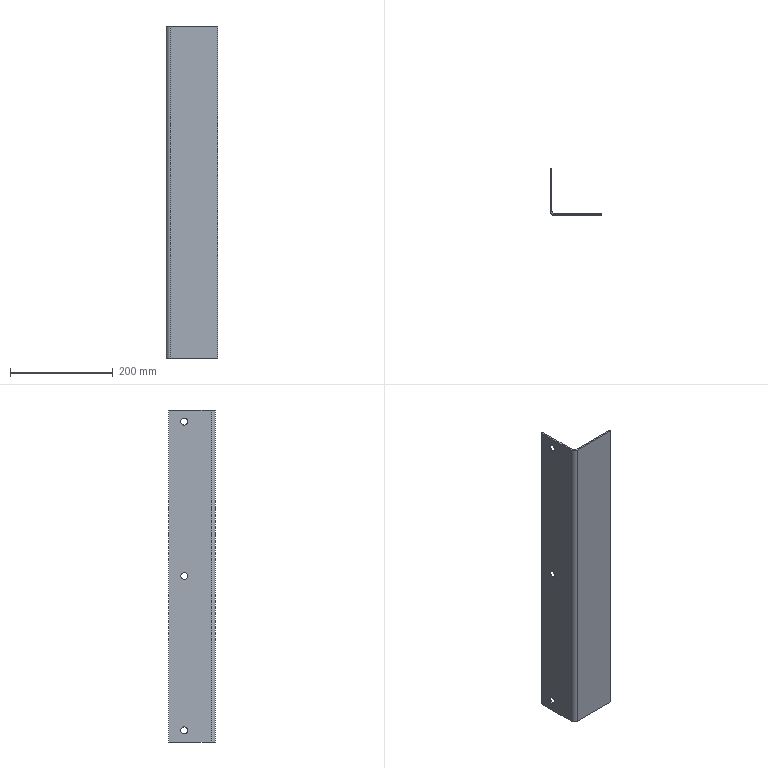Part | SolidWorks | features FlatPattern 1, ICE 1, SMBaseFlange 1, SheetMetal 1 | 1 solid | 20 faces | box 100 x 90 x 645 mm | volume 355061 mm3 | plane 12 | cylinder 8 | commonest cylinder face diameters 14 x6 10 x1 16 x1
STEP:
#1=CARTESIAN_POINT('',(0.,67.,300.));
#2=VERTEX_POINT('',#1);
#3=CARTESIAN_POINT('',(0.,53.,300.));
#4=VERTEX_POINT('',#3);
#5=CARTESIAN_POINT('',(0.,60.,300.));
#6=DIRECTION('',(-1.,0.,0.));
#7=DIRECTION('',(0.,-1.,0.));
#8=AXIS2_PLACEMENT_3D('',#5,#6,#7);
#9=CIRCLE('',#8,7.);
#10=EDGE_CURVE('',#2,#4,#9,.T.);
#11=ORIENTED_EDGE('',*,*,#10,.T.);
#12=CARTESIAN_POINT('',(3.,53.,300.));
#13=VERTEX_POINT('',#12);
#14=CARTESIAN_POINT('',(-7.,53.,300.));
#15=DIRECTION('',(1.,0.,0.));
#16=VECTOR('',#15,1000.);
#17=LINE('',#14,#16);
#18=EDGE_CURVE('',#4,#13,#17,.T.);
#19=ORIENTED_EDGE('',*,*,#18,.T.);
#20=CARTESIAN_POINT('',(3.,67.,300.));
#21=VERTEX_POINT('',#20);
#22=CARTESIAN_POINT('',(3.,60.,300.));
#23=DIRECTION('',(1.,0.,0.));
#24=DIRECTION('',(0.,1.,0.));
#25=AXIS2_PLACEMENT_3D('',#22,#23,#24);
#26=CIRCLE('',#25,7.);
#27=EDGE_CURVE('',#13,#21,#26,.T.);
#28=ORIENTED_EDGE('',*,*,#27,.T.);
#29=CARTESIAN_POINT('',(-7.,67.,300.));
#30=DIRECTION('',(1.,0.,0.));
#31=VECTOR('',#30,1000.);
#32=LINE('',#29,#31);
#33=EDGE_CURVE('',#2,#21,#32,.T.);
#34=ORIENTED_EDGE('',*,*,#33,.F.);
#35=EDGE_LOOP('',(#11,#19,#28,#34));
#36=FACE_OUTER_BOUND('',#35,.T.);
#37=CARTESIAN_POINT('',(-7.,60.,300.));
#38=DIRECTION('',(1.,0.,0.));
#39=DIRECTION('',(0.,1.,0.));
#40=AXIS2_PLACEMENT_3D('',#37,#38,#39);
#41=CYLINDRICAL_SURFACE('',#40,7.);
#42=ADVANCED_FACE('',(#36),#41,.F.);
#43=CARTESIAN_POINT('',(0.,67.,-300.));
#44=VERTEX_POINT('',#43);
#45=CARTESIAN_POINT('',(0.,53.,-300.));
#46=VERTEX_POINT('',#45);
#47=CARTESIAN_POINT('',(0.,60.,-300.));
#48=DIRECTION('',(-1.,0.,0.));
#49=DIRECTION('',(0.,-1.,0.));
#50=AXIS2_PLACEMENT_3D('',#47,#48,#49);
#51=CIRCLE('',#50,7.);
#52=EDGE_CURVE('',#44,#46,#51,.T.);
#53=ORIENTED_EDGE('',*,*,#52,.T.);
#54=CARTESIAN_POINT('',(3.,53.,-300.));
#55=VERTEX_POINT('',#54);
#56=CARTESIAN_POINT('',(-7.,53.,-300.));
#57=DIRECTION('',(1.,0.,0.));
#58=VECTOR('',#57,1000.);
#59=LINE('',#56,#58);
#60=EDGE_CURVE('',#46,#55,#59,.T.);
#61=ORIENTED_EDGE('',*,*,#60,.T.);
#62=CARTESIAN_POINT('',(3.,67.,-300.));
#63=VERTEX_POINT('',#62);
#64=CARTESIAN_POINT('',(3.,60.,-300.));
#65=DIRECTION('',(1.,0.,0.));
#66=DIRECTION('',(0.,1.,0.));
#67=AXIS2_PLACEMENT_3D('',#64,#65,#66);
#68=CIRCLE('',#67,7.);
#69=EDGE_CURVE('',#55,#63,#68,.T.);
#70=ORIENTED_EDGE('',*,*,#69,.T.);
#71=CARTESIAN_POINT('',(-7.,67.,-300.));
#72=DIRECTION('',(1.,0.,0.));
#73=VECTOR('',#72,1000.);
#74=LINE('',#71,#73);
#75=EDGE_CURVE('',#44,#63,#74,.T.);
#76=ORIENTED_EDGE('',*,*,#75,.F.);
#77=EDGE_LOOP('',(#53,#61,#70,#76));
#78=FACE_OUTER_BOUND('',#77,.T.);
#79=CARTESIAN_POINT('',(-7.,60.,-300.));
#80=DIRECTION('',(1.,0.,0.));
#81=DIRECTION('',(0.,1.,0.));
#82=AXIS2_PLACEMENT_3D('',#79,#80,#81);
#83=CYLINDRICAL_SURFACE('',#82,7.);
#84=ADVANCED_FACE('',(#78),#83,.F.);
#85=CARTESIAN_POINT('',(0.,67.,0.));
#86=VERTEX_POINT('',#85);
#87=CARTESIAN_POINT('',(0.,53.,0.));
#88=VERTEX_POINT('',#87);
#89=CARTESIAN_POINT('',(0.,60.,0.));
#90=DIRECTION('',(-1.,0.,0.));
#91=DIRECTION('',(0.,-1.,0.));
#92=AXIS2_PLACEMENT_3D('',#89,#90,#91);
#93=CIRCLE('',#92,7.);
#94=EDGE_CURVE('',#86,#88,#93,.T.);
#95=ORIENTED_EDGE('',*,*,#94,.T.);
#96=CARTESIAN_POINT('',(3.,53.,0.));
#97=VERTEX_POINT('',#96);
#98=CARTESIAN_POINT('',(-7.,53.,0.));
#99=DIRECTION('',(1.,0.,0.));
#100=VECTOR('',#99,1000.);
#101=LINE('',#98,#100);
#102=EDGE_CURVE('',#88,#97,#101,.T.);
#103=ORIENTED_EDGE('',*,*,#102,.T.);
#104=CARTESIAN_POINT('',(3.,67.,0.));
#105=VERTEX_POINT('',#104);
#106=CARTESIAN_POINT('',(3.,60.,0.));
#107=DIRECTION('',(1.,0.,0.));
#108=DIRECTION('',(0.,1.,0.));
#109=AXIS2_PLACEMENT_3D('',#106,#107,#108);
#110=CIRCLE('',#109,7.);
#111=EDGE_CURVE('',#97,#105,#110,.T.);
#112=ORIENTED_EDGE('',*,*,#111,.T.);
#113=CARTESIAN_POINT('',(-7.,67.,0.));
#114=DIRECTION('',(1.,0.,0.));
#115=VECTOR('',#114,1000.);
#116=LINE('',#113,#115);
#117=EDGE_CURVE('',#86,#105,#116,.T.);
#118=ORIENTED_EDGE('',*,*,#117,.F.);
#119=EDGE_LOOP('',(#95,#103,#112,#118));
#120=FACE_OUTER_BOUND('',#119,.T.);
#121=CARTESIAN_POINT('',(-7.,60.,0.));
#122=DIRECTION('',(1.,0.,0.));
#123=DIRECTION('',(0.,1.,0.));
#124=AXIS2_PLACEMENT_3D('',#121,#122,#123);
#125=CYLINDRICAL_SURFACE('',#124,7.);
#126=ADVANCED_FACE('',(#120),#125,.F.);
#127=CARTESIAN_POINT('',(0.,8.,322.5));
#128=VERTEX_POINT('',#127);
#129=CARTESIAN_POINT('',(3.,8.,322.5));
#130=VERTEX_POINT('',#129);
#131=CARTESIAN_POINT('',(0.,8.,322.5));
#132=DIRECTION('',(1.,0.,0.));
#133=VECTOR('',#132,1000.);
#134=LINE('',#131,#133);
#135=EDGE_CURVE('',#128,#130,#134,.T.);
#136=ORIENTED_EDGE('',*,*,#135,.F.);
#137=CARTESIAN_POINT('',(8.,0.,322.5));
#138=VERTEX_POINT('',#137);
#139=CARTESIAN_POINT('',(8.,8.,322.5));
#140=DIRECTION('',(0.,0.,-1.));
#141=DIRECTION('',(1.,0.,0.));
#142=AXIS2_PLACEMENT_3D('',#139,#140,#141);
#143=CIRCLE('',#142,8.);
#144=EDGE_CURVE('',#138,#128,#143,.T.);
#145=ORIENTED_EDGE('',*,*,#144,.F.);
#146=CARTESIAN_POINT('',(8.,3.,322.5));
#147=VERTEX_POINT('',#146);
#148=CARTESIAN_POINT('',(8.,3.,322.5));
#149=DIRECTION('',(0.,-1.,0.));
#150=VECTOR('',#149,1000.);
#151=LINE('',#148,#150);
#152=EDGE_CURVE('',#147,#138,#151,.T.);
#153=ORIENTED_EDGE('',*,*,#152,.F.);
#154=CARTESIAN_POINT('',(8.,8.,322.5));
#155=DIRECTION('',(0.,0.,-1.));
#156=DIRECTION('',(1.,0.,0.));
#157=AXIS2_PLACEMENT_3D('',#154,#155,#156);
#158=CIRCLE('',#157,5.);
#159=EDGE_CURVE('',#147,#130,#158,.T.);
#160=ORIENTED_EDGE('',*,*,#159,.T.);
#161=EDGE_LOOP('',(#136,#145,#153,#160));
#162=FACE_OUTER_BOUND('',#161,.T.);
#163=CARTESIAN_POINT('',(0.,8.,322.5));
#164=DIRECTION('',(0.,0.,1.));
#165=DIRECTION('',(1.,0.,0.));
#166=AXIS2_PLACEMENT_3D('',#163,#164,#165);
#167=PLANE('',#166);
#168=ADVANCED_FACE('',(#162),#167,.T.);
#169=CARTESIAN_POINT('',(0.,90.,322.5));
#170=VERTEX_POINT('',#169);
#171=CARTESIAN_POINT('',(0.,0.,322.5));
#172=DIRECTION('',(0.,1.,0.));
#173=VECTOR('',#172,1000.);
#174=LINE('',#171,#173);
#175=EDGE_CURVE('',#128,#170,#174,.T.);
#176=ORIENTED_EDGE('',*,*,#175,.F.);
#177=ORIENTED_EDGE('',*,*,#135,.T.);
#178=CARTESIAN_POINT('',(3.,90.,322.5));
#179=VERTEX_POINT('',#178);
#180=CARTESIAN_POINT('',(3.,0.,322.5));
#181=DIRECTION('',(0.,1.,0.));
#182=VECTOR('',#181,1000.);
#183=LINE('',#180,#182);
#184=EDGE_CURVE('',#130,#179,#183,.T.);
#185=ORIENTED_EDGE('',*,*,#184,.T.);
#186=CARTESIAN_POINT('',(0.,90.,322.5));
#187=DIRECTION('',(1.,0.,0.));
#188=VECTOR('',#187,1000.);
#189=LINE('',#186,#188);
#190=EDGE_CURVE('',#170,#179,#189,.T.);
#191=ORIENTED_EDGE('',*,*,#190,.F.);
#192=EDGE_LOOP('',(#176,#177,#185,#191));
#193=FACE_OUTER_BOUND('',#192,.T.);
#194=CARTESIAN_POINT('',(8.,3.,322.5));
#195=DIRECTION('',(0.,0.,1.));
#196=DIRECTION('',(1.,0.,0.));
#197=AXIS2_PLACEMENT_3D('',#194,#195,#196);
#198=PLANE('',#197);
#199=ADVANCED_FACE('',(#193),#198,.T.);
#200=CARTESIAN_POINT('',(8.,0.,-322.5));
#201=VERTEX_POINT('',#200);
#202=CARTESIAN_POINT('',(8.,3.,-322.5));
#203=VERTEX_POINT('',#202);
#204=CARTESIAN_POINT('',(8.,0.,-322.5));
#205=DIRECTION('',(0.,1.,0.));
#206=VECTOR('',#205,1000.);
#207=LINE('',#204,#206);
#208=EDGE_CURVE('',#201,#203,#207,.T.);
#209=ORIENTED_EDGE('',*,*,#208,.F.);
#210=CARTESIAN_POINT('',(0.,8.,-322.5));
#211=VERTEX_POINT('',#210);
#212=CARTESIAN_POINT('',(8.,8.,-322.5));
#213=DIRECTION('',(0.,0.,-1.));
#214=DIRECTION('',(1.,0.,0.));
#215=AXIS2_PLACEMENT_3D('',#212,#213,#214);
#216=CIRCLE('',#215,8.);
#217=EDGE_CURVE('',#201,#211,#216,.T.);
#218=ORIENTED_EDGE('',*,*,#217,.T.);
#219=CARTESIAN_POINT('',(3.,8.,-322.5));
#220=VERTEX_POINT('',#219);
#221=CARTESIAN_POINT('',(3.,8.,-322.5));
#222=DIRECTION('',(-1.,0.,0.));
#223=VECTOR('',#222,1000.);
#224=LINE('',#221,#223);
#225=EDGE_CURVE('',#220,#211,#224,.T.);
#226=ORIENTED_EDGE('',*,*,#225,.F.);
#227=CARTESIAN_POINT('',(8.,8.,-322.5));
#228=DIRECTION('',(0.,0.,-1.));
#229=DIRECTION('',(1.,0.,0.));
#230=AXIS2_PLACEMENT_3D('',#227,#228,#229);
#231=CIRCLE('',#230,5.);
#232=EDGE_CURVE('',#203,#220,#231,.T.);
#233=ORIENTED_EDGE('',*,*,#232,.F.);
#234=EDGE_LOOP('',(#209,#218,#226,#233));
#235=FACE_OUTER_BOUND('',#234,.T.);
#236=CARTESIAN_POINT('',(8.,0.,-322.5));
#237=DIRECTION('',(0.,0.,-1.));
#238=DIRECTION('',(-1.,0.,0.));
#239=AXIS2_PLACEMENT_3D('',#236,#237,#238);
#240=PLANE('',#239);
#241=ADVANCED_FACE('',(#235),#240,.T.);
#242=CARTESIAN_POINT('',(100.,0.,-322.5));
#243=VERTEX_POINT('',#242);
#244=CARTESIAN_POINT('',(100.,0.,-322.5));
#245=DIRECTION('',(-1.,0.,0.));
#246=VECTOR('',#245,1000.);
#247=LINE('',#244,#246);
#248=EDGE_CURVE('',#243,#201,#247,.T.);
#249=ORIENTED_EDGE('',*,*,#248,.T.);
#250=ORIENTED_EDGE('',*,*,#208,.T.);
#251=CARTESIAN_POINT('',(100.,3.,-322.5));
#252=VERTEX_POINT('',#251);
#253=CARTESIAN_POINT('',(100.,3.,-322.5));
#254=DIRECTION('',(-1.,0.,0.));
#255=VECTOR('',#254,1000.);
#256=LINE('',#253,#255);
#257=EDGE_CURVE('',#252,#203,#256,.T.);
#258=ORIENTED_EDGE('',*,*,#257,.F.);
#259=CARTESIAN_POINT('',(100.,3.,-322.5));
#260=DIRECTION('',(0.,-1.,0.));
#261=VECTOR('',#260,1000.);
#262=LINE('',#259,#261);
#263=EDGE_CURVE('',#252,#243,#262,.T.);
#264=ORIENTED_EDGE('',*,*,#263,.T.);
#265=EDGE_LOOP('',(#249,#250,#258,#264));
#266=FACE_OUTER_BOUND('',#265,.T.);
#267=CARTESIAN_POINT('',(3.,8.,-322.5));
#268=DIRECTION('',(0.,0.,-1.));
#269=DIRECTION('',(-1.,0.,0.));
#270=AXIS2_PLACEMENT_3D('',#267,#268,#269);
#271=PLANE('',#270);
#272=ADVANCED_FACE('',(#266),#271,.T.);
#273=CARTESIAN_POINT('',(3.,60.,300.));
#274=DIRECTION('',(1.,0.,0.));
#275=DIRECTION('',(0.,1.,0.));
#276=AXIS2_PLACEMENT_3D('',#273,#274,#275);
#277=CIRCLE('',#276,7.);
#278=EDGE_CURVE('',#21,#13,#277,.T.);
#279=ORIENTED_EDGE('',*,*,#278,.F.);
#280=ORIENTED_EDGE('',*,*,#27,.F.);
#281=EDGE_LOOP('',(#279,#280));
#282=FACE_BOUND('',#281,.T.);
#283=CARTESIAN_POINT('',(3.,60.,-300.));
#284=DIRECTION('',(1.,0.,0.));
#285=DIRECTION('',(0.,1.,0.));
#286=AXIS2_PLACEMENT_3D('',#283,#284,#285);
#287=CIRCLE('',#286,7.);
#288=EDGE_CURVE('',#63,#55,#287,.T.);
#289=ORIENTED_EDGE('',*,*,#288,.F.);
#290=ORIENTED_EDGE('',*,*,#69,.F.);
#291=EDGE_LOOP('',(#289,#290));
#292=FACE_BOUND('',#291,.T.);
#293=CARTESIAN_POINT('',(3.,60.,0.));
#294=DIRECTION('',(1.,0.,0.));
#295=DIRECTION('',(0.,1.,0.));
#296=AXIS2_PLACEMENT_3D('',#293,#294,#295);
#297=CIRCLE('',#296,7.);
#298=EDGE_CURVE('',#105,#97,#297,.T.);
#299=ORIENTED_EDGE('',*,*,#298,.F.);
#300=ORIENTED_EDGE('',*,*,#111,.F.);
#301=EDGE_LOOP('',(#299,#300));
#302=FACE_BOUND('',#301,.T.);
#303=CARTESIAN_POINT('',(3.,90.,-322.5));
#304=VERTEX_POINT('',#303);
#305=CARTESIAN_POINT('',(3.,0.,-322.5));
#306=DIRECTION('',(0.,1.,0.));
#307=VECTOR('',#306,1000.);
#308=LINE('',#305,#307);
#309=EDGE_CURVE('',#220,#304,#308,.T.);
#310=ORIENTED_EDGE('',*,*,#309,.T.);
#311=CARTESIAN_POINT('',(3.,90.,322.5));
#312=DIRECTION('',(0.,0.,-1.));
#313=VECTOR('',#312,1000.);
#314=LINE('',#311,#313);
#315=EDGE_CURVE('',#179,#304,#314,.T.);
#316=ORIENTED_EDGE('',*,*,#315,.F.);
#317=ORIENTED_EDGE('',*,*,#184,.F.);
#318=CARTESIAN_POINT('',(3.,8.,322.5));
#319=DIRECTION('',(0.,0.,-1.));
#320=VECTOR('',#319,1000.);
#321=LINE('',#318,#320);
#322=EDGE_CURVE('',#130,#220,#321,.T.);
#323=ORIENTED_EDGE('',*,*,#322,.T.);
#324=EDGE_LOOP('',(#310,#316,#317,#323));
#325=FACE_OUTER_BOUND('',#324,.T.);
#326=CARTESIAN_POINT('',(3.,0.,322.5));
#327=DIRECTION('',(-1.,0.,0.));
#328=DIRECTION('',(0.,-1.,0.));
#329=AXIS2_PLACEMENT_3D('',#326,#327,#328);
#330=PLANE('',#329);
#331=ADVANCED_FACE('',(#282,#292,#302,#325),#330,.F.);
#332=CARTESIAN_POINT('',(0.,90.,-322.5));
#333=VERTEX_POINT('',#332);
#334=CARTESIAN_POINT('',(0.,90.,-322.5));
#335=DIRECTION('',(1.,0.,0.));
#336=VECTOR('',#335,1000.);
#337=LINE('',#334,#336);
#338=EDGE_CURVE('',#333,#304,#337,.T.);
#339=ORIENTED_EDGE('',*,*,#338,.F.);
#340=CARTESIAN_POINT('',(0.,90.,322.5));
#341=DIRECTION('',(0.,0.,-1.));
#342=VECTOR('',#341,1000.);
#343=LINE('',#340,#342);
#344=EDGE_CURVE('',#170,#333,#343,.T.);
#345=ORIENTED_EDGE('',*,*,#344,.F.);
#346=ORIENTED_EDGE('',*,*,#190,.T.);
#347=ORIENTED_EDGE('',*,*,#315,.T.);
#348=EDGE_LOOP('',(#339,#345,#346,#347));
#349=FACE_OUTER_BOUND('',#348,.T.);
#350=CARTESIAN_POINT('',(0.,90.,322.5));
#351=DIRECTION('',(0.,1.,0.));
#352=DIRECTION('',(-1.,0.,0.));
#353=AXIS2_PLACEMENT_3D('',#350,#351,#352);
#354=PLANE('',#353);
#355=ADVANCED_FACE('',(#349),#354,.T.);
#356=ORIENTED_EDGE('',*,*,#10,.F.);
#357=CARTESIAN_POINT('',(0.,60.,300.));
#358=DIRECTION('',(-1.,0.,0.));
#359=DIRECTION('',(0.,-1.,0.));
#360=AXIS2_PLACEMENT_3D('',#357,#358,#359);
#361=CIRCLE('',#360,7.);
#362=EDGE_CURVE('',#4,#2,#361,.T.);
#363=ORIENTED_EDGE('',*,*,#362,.F.);
#364=EDGE_LOOP('',(#356,#363));
#365=FACE_BOUND('',#364,.T.);
#366=ORIENTED_EDGE('',*,*,#52,.F.);
#367=CARTESIAN_POINT('',(0.,60.,-300.));
#368=DIRECTION('',(-1.,0.,0.));
#369=DIRECTION('',(0.,-1.,0.));
#370=AXIS2_PLACEMENT_3D('',#367,#368,#369);
#371=CIRCLE('',#370,7.);
#372=EDGE_CURVE('',#46,#44,#371,.T.);
#373=ORIENTED_EDGE('',*,*,#372,.F.);
#374=EDGE_LOOP('',(#366,#373));
#375=FACE_BOUND('',#374,.T.);
#376=ORIENTED_EDGE('',*,*,#94,.F.);
#377=CARTESIAN_POINT('',(0.,60.,0.));
#378=DIRECTION('',(-1.,0.,0.));
#379=DIRECTION('',(0.,-1.,0.));
#380=AXIS2_PLACEMENT_3D('',#377,#378,#379);
#381=CIRCLE('',#380,7.);
#382=EDGE_CURVE('',#88,#86,#381,.T.);
#383=ORIENTED_EDGE('',*,*,#382,.F.);
#384=EDGE_LOOP('',(#376,#383));
#385=FACE_BOUND('',#384,.T.);
#386=CARTESIAN_POINT('',(0.,0.,-322.5));
#387=DIRECTION('',(0.,1.,0.));
#388=VECTOR('',#387,1000.);
#389=LINE('',#386,#388);
#390=EDGE_CURVE('',#211,#333,#389,.T.);
#391=ORIENTED_EDGE('',*,*,#390,.F.);
#392=CARTESIAN_POINT('',(0.,8.,322.5));
#393=DIRECTION('',(0.,0.,-1.));
#394=VECTOR('',#393,1000.);
#395=LINE('',#392,#394);
#396=EDGE_CURVE('',#128,#211,#395,.T.);
#397=ORIENTED_EDGE('',*,*,#396,.F.);
#398=ORIENTED_EDGE('',*,*,#175,.T.);
#399=ORIENTED_EDGE('',*,*,#344,.T.);
#400=EDGE_LOOP('',(#391,#397,#398,#399));
#401=FACE_OUTER_BOUND('',#400,.T.);
#402=CARTESIAN_POINT('',(0.,0.,322.5));
#403=DIRECTION('',(-1.,0.,0.));
#404=DIRECTION('',(0.,-1.,0.));
#405=AXIS2_PLACEMENT_3D('',#402,#403,#404);
#406=PLANE('',#405);
#407=ADVANCED_FACE('',(#365,#375,#385,#401),#406,.T.);
#408=ORIENTED_EDGE('',*,*,#217,.F.);
#409=CARTESIAN_POINT('',(8.,0.,322.5));
#410=DIRECTION('',(0.,0.,-1.));
#411=VECTOR('',#410,1000.);
#412=LINE('',#409,#411);
#413=EDGE_CURVE('',#138,#201,#412,.T.);
#414=ORIENTED_EDGE('',*,*,#413,.F.);
#415=ORIENTED_EDGE('',*,*,#144,.T.);
#416=ORIENTED_EDGE('',*,*,#396,.T.);
#417=EDGE_LOOP('',(#408,#414,#415,#416));
#418=FACE_OUTER_BOUND('',#417,.T.);
#419=CARTESIAN_POINT('',(8.,8.,322.5));
#420=DIRECTION('',(0.,0.,-1.));
#421=DIRECTION('',(-1.,0.,0.));
#422=AXIS2_PLACEMENT_3D('',#419,#420,#421);
#423=CYLINDRICAL_SURFACE('',#422,8.);
#424=ADVANCED_FACE('',(#418),#423,.T.);
#425=ORIENTED_EDGE('',*,*,#248,.F.);
#426=CARTESIAN_POINT('',(100.,0.,322.5));
#427=VERTEX_POINT('',#426);
#428=CARTESIAN_POINT('',(100.,0.,322.5));
#429=DIRECTION('',(0.,0.,-1.));
#430=VECTOR('',#429,1000.);
#431=LINE('',#428,#430);
#432=EDGE_CURVE('',#427,#243,#431,.T.);
#433=ORIENTED_EDGE('',*,*,#432,.F.);
#434=CARTESIAN_POINT('',(100.,0.,322.5));
#435=DIRECTION('',(-1.,0.,0.));
#436=VECTOR('',#435,1000.);
#437=LINE('',#434,#436);
#438=EDGE_CURVE('',#427,#138,#437,.T.);
#439=ORIENTED_EDGE('',*,*,#438,.T.);
#440=ORIENTED_EDGE('',*,*,#413,.T.);
#441=EDGE_LOOP('',(#425,#433,#439,#440));
#442=FACE_OUTER_BOUND('',#441,.T.);
#443=CARTESIAN_POINT('',(100.,0.,322.5));
#444=DIRECTION('',(0.,-1.,0.));
#445=DIRECTION('',(1.,0.,0.));
#446=AXIS2_PLACEMENT_3D('',#443,#444,#445);
#447=PLANE('',#446);
#448=ADVANCED_FACE('',(#442),#447,.T.);
#449=ORIENTED_EDGE('',*,*,#263,.F.);
#450=CARTESIAN_POINT('',(100.,3.,322.5));
#451=VERTEX_POINT('',#450);
#452=CARTESIAN_POINT('',(100.,3.,322.5));
#453=DIRECTION('',(0.,0.,-1.));
#454=VECTOR('',#453,1000.);
#455=LINE('',#452,#454);
#456=EDGE_CURVE('',#451,#252,#455,.T.);
#457=ORIENTED_EDGE('',*,*,#456,.F.);
#458=CARTESIAN_POINT('',(100.,3.,322.5));
#459=DIRECTION('',(0.,-1.,0.));
#460=VECTOR('',#459,1000.);
#461=LINE('',#458,#460);
#462=EDGE_CURVE('',#451,#427,#461,.T.);
#463=ORIENTED_EDGE('',*,*,#462,.T.);
#464=ORIENTED_EDGE('',*,*,#432,.T.);
#465=EDGE_LOOP('',(#449,#457,#463,#464));
#466=FACE_OUTER_BOUND('',#465,.T.);
#467=CARTESIAN_POINT('',(100.,3.,322.5));
#468=DIRECTION('',(1.,0.,0.));
#469=DIRECTION('',(0.,0.,-1.));
#470=AXIS2_PLACEMENT_3D('',#467,#468,#469);
#471=PLANE('',#470);
#472=ADVANCED_FACE('',(#466),#471,.T.);
#473=ORIENTED_EDGE('',*,*,#257,.T.);
#474=CARTESIAN_POINT('',(8.,3.,322.5));
#475=DIRECTION('',(0.,0.,-1.));
#476=VECTOR('',#475,1000.);
#477=LINE('',#474,#476);
#478=EDGE_CURVE('',#147,#203,#477,.T.);
#479=ORIENTED_EDGE('',*,*,#478,.F.);
#480=CARTESIAN_POINT('',(100.,3.,322.5));
#481=DIRECTION('',(-1.,0.,0.));
#482=VECTOR('',#481,1000.);
#483=LINE('',#480,#482);
#484=EDGE_CURVE('',#451,#147,#483,.T.);
#485=ORIENTED_EDGE('',*,*,#484,.F.);
#486=ORIENTED_EDGE('',*,*,#456,.T.);
#487=EDGE_LOOP('',(#473,#479,#485,#486));
#488=FACE_OUTER_BOUND('',#487,.T.);
#489=CARTESIAN_POINT('',(100.,3.,322.5));
#490=DIRECTION('',(0.,-1.,0.));
#491=DIRECTION('',(1.,0.,0.));
#492=AXIS2_PLACEMENT_3D('',#489,#490,#491);
#493=PLANE('',#492);
#494=ADVANCED_FACE('',(#488),#493,.F.);
#495=ORIENTED_EDGE('',*,*,#232,.T.);
#496=ORIENTED_EDGE('',*,*,#322,.F.);
#497=ORIENTED_EDGE('',*,*,#159,.F.);
#498=ORIENTED_EDGE('',*,*,#478,.T.);
#499=EDGE_LOOP('',(#495,#496,#497,#498));
#500=FACE_OUTER_BOUND('',#499,.T.);
#501=CARTESIAN_POINT('',(8.,8.,322.5));
#502=DIRECTION('',(0.,0.,-1.));
#503=DIRECTION('',(-1.,0.,0.));
#504=AXIS2_PLACEMENT_3D('',#501,#502,#503);
#505=CYLINDRICAL_SURFACE('',#504,5.);
#506=ADVANCED_FACE('',(#500),#505,.F.);
#507=ORIENTED_EDGE('',*,*,#484,.T.);
#508=ORIENTED_EDGE('',*,*,#152,.T.);
#509=ORIENTED_EDGE('',*,*,#438,.F.);
#510=ORIENTED_EDGE('',*,*,#462,.F.);
#511=EDGE_LOOP('',(#507,#508,#509,#510));
#512=FACE_OUTER_BOUND('',#511,.T.);
#513=CARTESIAN_POINT('',(8.,8.,322.5));
#514=DIRECTION('',(0.,0.,1.));
#515=DIRECTION('',(1.,0.,0.));
#516=AXIS2_PLACEMENT_3D('',#513,#514,#515);
#517=PLANE('',#516);
#518=ADVANCED_FACE('',(#512),#517,.T.);
#519=ORIENTED_EDGE('',*,*,#309,.F.);
#520=ORIENTED_EDGE('',*,*,#225,.T.);
#521=ORIENTED_EDGE('',*,*,#390,.T.);
#522=ORIENTED_EDGE('',*,*,#338,.T.);
#523=EDGE_LOOP('',(#519,#520,#521,#522));
#524=FACE_OUTER_BOUND('',#523,.T.);
#525=CARTESIAN_POINT('',(8.,8.,-322.5));
#526=DIRECTION('',(0.,0.,1.));
#527=DIRECTION('',(1.,0.,0.));
#528=AXIS2_PLACEMENT_3D('',#525,#526,#527);
#529=PLANE('',#528);
#530=ADVANCED_FACE('',(#524),#529,.F.);
#531=ORIENTED_EDGE('',*,*,#102,.F.);
#532=ORIENTED_EDGE('',*,*,#382,.T.);
#533=ORIENTED_EDGE('',*,*,#117,.T.);
#534=ORIENTED_EDGE('',*,*,#298,.T.);
#535=EDGE_LOOP('',(#531,#532,#533,#534));
#536=FACE_OUTER_BOUND('',#535,.T.);
#537=CARTESIAN_POINT('',(-7.,60.,0.));
#538=DIRECTION('',(1.,0.,0.));
#539=DIRECTION('',(0.,1.,0.));
#540=AXIS2_PLACEMENT_3D('',#537,#538,#539);
#541=CYLINDRICAL_SURFACE('',#540,7.);
#542=ADVANCED_FACE('',(#536),#541,.F.);
#543=ORIENTED_EDGE('',*,*,#60,.F.);
#544=ORIENTED_EDGE('',*,*,#372,.T.);
#545=ORIENTED_EDGE('',*,*,#75,.T.);
#546=ORIENTED_EDGE('',*,*,#288,.T.);
#547=EDGE_LOOP('',(#543,#544,#545,#546));
#548=FACE_OUTER_BOUND('',#547,.T.);
#549=CARTESIAN_POINT('',(-7.,60.,-300.));
#550=DIRECTION('',(1.,0.,0.));
#551=DIRECTION('',(0.,1.,0.));
#552=AXIS2_PLACEMENT_3D('',#549,#550,#551);
#553=CYLINDRICAL_SURFACE('',#552,7.);
#554=ADVANCED_FACE('',(#548),#553,.F.);
#555=ORIENTED_EDGE('',*,*,#18,.F.);
#556=ORIENTED_EDGE('',*,*,#362,.T.);
#557=ORIENTED_EDGE('',*,*,#33,.T.);
#558=ORIENTED_EDGE('',*,*,#278,.T.);
#559=EDGE_LOOP('',(#555,#556,#557,#558));
#560=FACE_OUTER_BOUND('',#559,.T.);
#561=CARTESIAN_POINT('',(-7.,60.,300.));
#562=DIRECTION('',(1.,0.,0.));
#563=DIRECTION('',(0.,1.,0.));
#564=AXIS2_PLACEMENT_3D('',#561,#562,#563);
#565=CYLINDRICAL_SURFACE('',#564,7.);
#566=ADVANCED_FACE('',(#560),#565,.F.);
#567=CLOSED_SHELL('',(#42,#84,#126,#168,#199,#241,#272,#331,#355,#407,#424,#448,#472,#494,#506,#518,#530,#542,#554,#566));
#568=MANIFOLD_SOLID_BREP('',#567);
#569=CARTESIAN_POINT('',(0.,0.,0.));
#570=DIRECTION('',(0.,0.,1.));
#571=DIRECTION('',(1.,0.,0.));
#572=AXIS2_PLACEMENT_3D('',#569,#570,#571);
#573=(LENGTH_UNIT()NAMED_UNIT(*)SI_UNIT(.MILLI.,.METRE.));
#574=UNCERTAINTY_MEASURE_WITH_UNIT(LENGTH_MEASURE(0.00001),#573,'','');
#575=(NAMED_UNIT(*)PLANE_ANGLE_UNIT()SI_UNIT($,.RADIAN.));
#576=(NAMED_UNIT(*)SI_UNIT($,.STERADIAN.)SOLID_ANGLE_UNIT());
#577=(GEOMETRIC_REPRESENTATION_CONTEXT(3)GLOBAL_UNCERTAINTY_ASSIGNED_CONTEXT((#574))GLOBAL_UNIT_ASSIGNED_CONTEXT((#573,#575,#576))REPRESENTATION_CONTEXT('',''));
#578=ADVANCED_BREP_SHAPE_REPRESENTATION('',(#568,#572),#577);